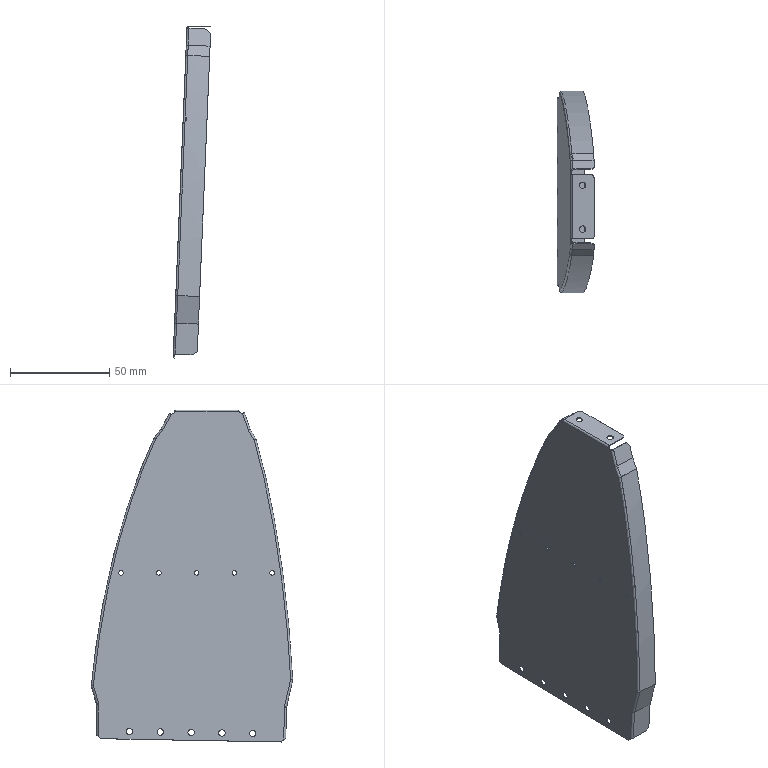Part | SolidWorks | features BaseBody 2 | 2 solids | 112 faces | box 18.995 x 101.225 x 166.89 mm | volume 9620 mm3 | cylinder 62 | plane 40 | spline 8 | cone 2 | commonest cylinder face diameters 2 x22 2.4 x20 3.2 x14 1 x2 3.108 x2 3.882 x2